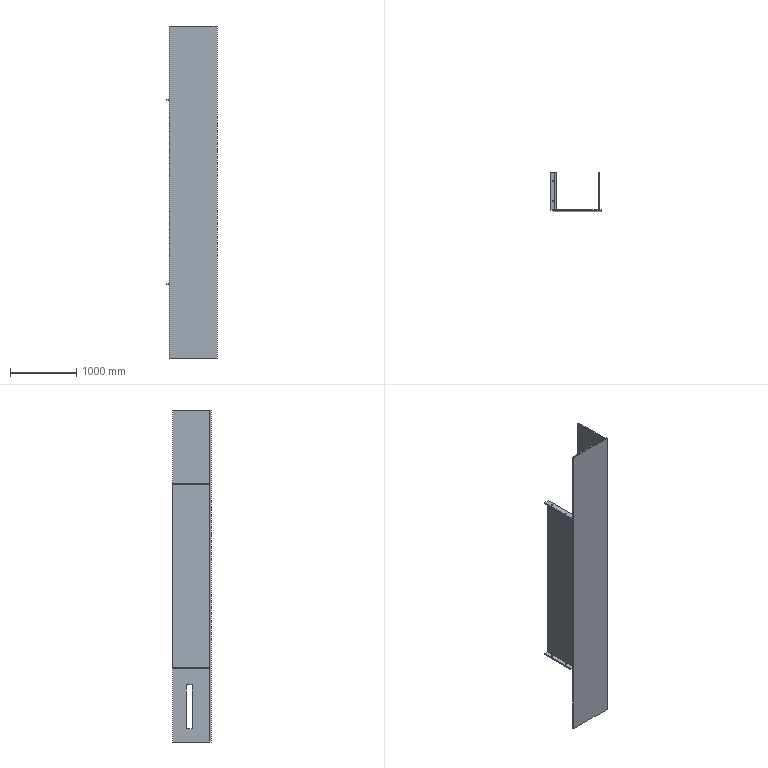Part | SolidWorks | features ICE 4, Extrusion 1 | 1 solid | 34 faces | box 755 x 580 x 5000 mm | volume 159485589 mm3 | plane 26 | cylinder 8 | commonest cylinder face diameters 22 x8
STEP:
#1=CARTESIAN_POINT('',(-376.,450.,3880.));
#2=VERTEX_POINT('',#1);
#3=CARTESIAN_POINT('',(-354.,450.,3880.));
#4=VERTEX_POINT('',#3);
#5=CARTESIAN_POINT('',(-365.,450.,3880.));
#6=DIRECTION('',(0.,0.,1.));
#7=DIRECTION('',(1.,0.,0.));
#8=AXIS2_PLACEMENT_3D('',#5,#6,#7);
#9=CIRCLE('',#8,11.);
#10=EDGE_CURVE('',#2,#4,#9,.T.);
#11=ORIENTED_EDGE('',*,*,#10,.F.);
#12=CARTESIAN_POINT('',(-376.,450.,3900.));
#13=VERTEX_POINT('',#12);
#14=CARTESIAN_POINT('',(-376.,450.,0.));
#15=DIRECTION('',(0.,0.,1.));
#16=VECTOR('',#15,1000.);
#17=LINE('',#14,#16);
#18=EDGE_CURVE('',#2,#13,#17,.T.);
#19=ORIENTED_EDGE('',*,*,#18,.T.);
#20=CARTESIAN_POINT('',(-354.,450.,3900.));
#21=VERTEX_POINT('',#20);
#22=CARTESIAN_POINT('',(-365.,450.,3900.));
#23=DIRECTION('',(0.,0.,1.));
#24=DIRECTION('',(1.,0.,0.));
#25=AXIS2_PLACEMENT_3D('',#22,#23,#24);
#26=CIRCLE('',#25,11.);
#27=EDGE_CURVE('',#13,#21,#26,.T.);
#28=ORIENTED_EDGE('',*,*,#27,.T.);
#29=CARTESIAN_POINT('',(-354.,450.,0.));
#30=DIRECTION('',(0.,0.,1.));
#31=VECTOR('',#30,1000.);
#32=LINE('',#29,#31);
#33=EDGE_CURVE('',#4,#21,#32,.T.);
#34=ORIENTED_EDGE('',*,*,#33,.F.);
#35=EDGE_LOOP('',(#11,#19,#28,#34));
#36=FACE_OUTER_BOUND('',#35,.T.);
#37=CARTESIAN_POINT('',(-365.,450.,0.));
#38=DIRECTION('',(0.,0.,1.));
#39=DIRECTION('',(1.,0.,0.));
#40=AXIS2_PLACEMENT_3D('',#37,#38,#39);
#41=CYLINDRICAL_SURFACE('',#40,11.);
#42=ADVANCED_FACE('',(#36),#41,.F.);
#43=CARTESIAN_POINT('',(-376.,150.,3880.));
#44=VERTEX_POINT('',#43);
#45=CARTESIAN_POINT('',(-354.,150.,3880.));
#46=VERTEX_POINT('',#45);
#47=CARTESIAN_POINT('',(-365.,150.,3880.));
#48=DIRECTION('',(0.,0.,1.));
#49=DIRECTION('',(1.,0.,0.));
#50=AXIS2_PLACEMENT_3D('',#47,#48,#49);
#51=CIRCLE('',#50,11.);
#52=EDGE_CURVE('',#44,#46,#51,.T.);
#53=ORIENTED_EDGE('',*,*,#52,.F.);
#54=CARTESIAN_POINT('',(-376.,150.,3900.));
#55=VERTEX_POINT('',#54);
#56=CARTESIAN_POINT('',(-376.,150.,0.));
#57=DIRECTION('',(0.,0.,1.));
#58=VECTOR('',#57,1000.);
#59=LINE('',#56,#58);
#60=EDGE_CURVE('',#44,#55,#59,.T.);
#61=ORIENTED_EDGE('',*,*,#60,.T.);
#62=CARTESIAN_POINT('',(-354.,150.,3900.));
#63=VERTEX_POINT('',#62);
#64=CARTESIAN_POINT('',(-365.,150.,3900.));
#65=DIRECTION('',(0.,0.,1.));
#66=DIRECTION('',(1.,0.,0.));
#67=AXIS2_PLACEMENT_3D('',#64,#65,#66);
#68=CIRCLE('',#67,11.);
#69=EDGE_CURVE('',#55,#63,#68,.T.);
#70=ORIENTED_EDGE('',*,*,#69,.T.);
#71=CARTESIAN_POINT('',(-354.,150.,0.));
#72=DIRECTION('',(0.,0.,1.));
#73=VECTOR('',#72,1000.);
#74=LINE('',#71,#73);
#75=EDGE_CURVE('',#46,#63,#74,.T.);
#76=ORIENTED_EDGE('',*,*,#75,.F.);
#77=EDGE_LOOP('',(#53,#61,#70,#76));
#78=FACE_OUTER_BOUND('',#77,.T.);
#79=CARTESIAN_POINT('',(-365.,150.,0.));
#80=DIRECTION('',(0.,0.,1.));
#81=DIRECTION('',(1.,0.,0.));
#82=AXIS2_PLACEMENT_3D('',#79,#80,#81);
#83=CYLINDRICAL_SURFACE('',#82,11.);
#84=ADVANCED_FACE('',(#78),#83,.F.);
#85=CARTESIAN_POINT('',(-376.,450.,1100.));
#86=VERTEX_POINT('',#85);
#87=CARTESIAN_POINT('',(-354.,450.,1100.));
#88=VERTEX_POINT('',#87);
#89=CARTESIAN_POINT('',(-365.,450.,1100.));
#90=DIRECTION('',(0.,0.,1.));
#91=DIRECTION('',(1.,0.,0.));
#92=AXIS2_PLACEMENT_3D('',#89,#90,#91);
#93=CIRCLE('',#92,11.);
#94=EDGE_CURVE('',#86,#88,#93,.T.);
#95=ORIENTED_EDGE('',*,*,#94,.F.);
#96=CARTESIAN_POINT('',(-376.,450.,1120.));
#97=VERTEX_POINT('',#96);
#98=CARTESIAN_POINT('',(-376.,450.,0.));
#99=DIRECTION('',(0.,0.,1.));
#100=VECTOR('',#99,1000.);
#101=LINE('',#98,#100);
#102=EDGE_CURVE('',#86,#97,#101,.T.);
#103=ORIENTED_EDGE('',*,*,#102,.T.);
#104=CARTESIAN_POINT('',(-354.,450.,1120.));
#105=VERTEX_POINT('',#104);
#106=CARTESIAN_POINT('',(-365.,450.,1120.));
#107=DIRECTION('',(0.,0.,-1.));
#108=DIRECTION('',(-1.,0.,0.));
#109=AXIS2_PLACEMENT_3D('',#106,#107,#108);
#110=CIRCLE('',#109,11.);
#111=EDGE_CURVE('',#105,#97,#110,.T.);
#112=ORIENTED_EDGE('',*,*,#111,.F.);
#113=CARTESIAN_POINT('',(-354.,450.,0.));
#114=DIRECTION('',(0.,0.,1.));
#115=VECTOR('',#114,1000.);
#116=LINE('',#113,#115);
#117=EDGE_CURVE('',#88,#105,#116,.T.);
#118=ORIENTED_EDGE('',*,*,#117,.F.);
#119=EDGE_LOOP('',(#95,#103,#112,#118));
#120=FACE_OUTER_BOUND('',#119,.T.);
#121=CARTESIAN_POINT('',(-365.,450.,0.));
#122=DIRECTION('',(0.,0.,1.));
#123=DIRECTION('',(1.,0.,0.));
#124=AXIS2_PLACEMENT_3D('',#121,#122,#123);
#125=CYLINDRICAL_SURFACE('',#124,11.);
#126=ADVANCED_FACE('',(#120),#125,.F.);
#127=CARTESIAN_POINT('',(-376.,150.,1100.));
#128=VERTEX_POINT('',#127);
#129=CARTESIAN_POINT('',(-354.,150.,1100.));
#130=VERTEX_POINT('',#129);
#131=CARTESIAN_POINT('',(-365.,150.,1100.));
#132=DIRECTION('',(0.,0.,1.));
#133=DIRECTION('',(1.,0.,0.));
#134=AXIS2_PLACEMENT_3D('',#131,#132,#133);
#135=CIRCLE('',#134,11.);
#136=EDGE_CURVE('',#128,#130,#135,.T.);
#137=ORIENTED_EDGE('',*,*,#136,.F.);
#138=CARTESIAN_POINT('',(-376.,150.,1120.));
#139=VERTEX_POINT('',#138);
#140=CARTESIAN_POINT('',(-376.,150.,0.));
#141=DIRECTION('',(0.,0.,1.));
#142=VECTOR('',#141,1000.);
#143=LINE('',#140,#142);
#144=EDGE_CURVE('',#128,#139,#143,.T.);
#145=ORIENTED_EDGE('',*,*,#144,.T.);
#146=CARTESIAN_POINT('',(-354.,150.,1120.));
#147=VERTEX_POINT('',#146);
#148=CARTESIAN_POINT('',(-365.,150.,1120.));
#149=DIRECTION('',(0.,0.,-1.));
#150=DIRECTION('',(-1.,0.,0.));
#151=AXIS2_PLACEMENT_3D('',#148,#149,#150);
#152=CIRCLE('',#151,11.);
#153=EDGE_CURVE('',#147,#139,#152,.T.);
#154=ORIENTED_EDGE('',*,*,#153,.F.);
#155=CARTESIAN_POINT('',(-354.,150.,0.));
#156=DIRECTION('',(0.,0.,1.));
#157=VECTOR('',#156,1000.);
#158=LINE('',#155,#157);
#159=EDGE_CURVE('',#130,#147,#158,.T.);
#160=ORIENTED_EDGE('',*,*,#159,.F.);
#161=EDGE_LOOP('',(#137,#145,#154,#160));
#162=FACE_OUTER_BOUND('',#161,.T.);
#163=CARTESIAN_POINT('',(-365.,150.,0.));
#164=DIRECTION('',(0.,0.,1.));
#165=DIRECTION('',(1.,0.,0.));
#166=AXIS2_PLACEMENT_3D('',#163,#164,#165);
#167=CYLINDRICAL_SURFACE('',#166,11.);
#168=ADVANCED_FACE('',(#162),#167,.F.);
#169=CARTESIAN_POINT('',(-335.,20.,1120.));
#170=VERTEX_POINT('',#169);
#171=CARTESIAN_POINT('',(-335.,580.,1120.));
#172=VERTEX_POINT('',#171);
#173=CARTESIAN_POINT('',(-335.,580.,1120.));
#174=DIRECTION('',(0.,1.,0.));
#175=VECTOR('',#174,1000.);
#176=LINE('',#173,#175);
#177=EDGE_CURVE('',#170,#172,#176,.T.);
#178=ORIENTED_EDGE('',*,*,#177,.F.);
#179=CARTESIAN_POINT('',(-335.,20.,3880.));
#180=VERTEX_POINT('',#179);
#181=CARTESIAN_POINT('',(-335.,20.,5000.));
#182=DIRECTION('',(0.,0.,-1.));
#183=VECTOR('',#182,1000.);
#184=LINE('',#181,#183);
#185=EDGE_CURVE('',#180,#170,#184,.T.);
#186=ORIENTED_EDGE('',*,*,#185,.F.);
#187=CARTESIAN_POINT('',(-335.,580.,3880.));
#188=VERTEX_POINT('',#187);
#189=CARTESIAN_POINT('',(-335.,580.,3880.));
#190=DIRECTION('',(0.,-1.,0.));
#191=VECTOR('',#190,1000.);
#192=LINE('',#189,#191);
#193=EDGE_CURVE('',#188,#180,#192,.T.);
#194=ORIENTED_EDGE('',*,*,#193,.F.);
#195=CARTESIAN_POINT('',(-335.,580.,5000.));
#196=DIRECTION('',(0.,0.,-1.));
#197=VECTOR('',#196,1000.);
#198=LINE('',#195,#197);
#199=EDGE_CURVE('',#188,#172,#198,.T.);
#200=ORIENTED_EDGE('',*,*,#199,.T.);
#201=EDGE_LOOP('',(#178,#186,#194,#200));
#202=FACE_OUTER_BOUND('',#201,.T.);
#203=CARTESIAN_POINT('',(-335.,20.,5000.));
#204=DIRECTION('',(1.,0.,0.));
#205=DIRECTION('',(0.,1.,0.));
#206=AXIS2_PLACEMENT_3D('',#203,#204,#205);
#207=PLANE('',#206);
#208=ADVANCED_FACE('',(#202),#207,.F.);
#209=CARTESIAN_POINT('',(-360.,20.,1100.));
#210=VERTEX_POINT('',#209);
#211=CARTESIAN_POINT('',(-360.,20.,0.));
#212=VERTEX_POINT('',#211);
#213=CARTESIAN_POINT('',(-360.,20.,5000.));
#214=DIRECTION('',(0.,0.,-1.));
#215=VECTOR('',#214,1000.);
#216=LINE('',#213,#215);
#217=EDGE_CURVE('',#210,#212,#216,.T.);
#218=ORIENTED_EDGE('',*,*,#217,.F.);
#219=CARTESIAN_POINT('',(-315.,20.,1100.));
#220=VERTEX_POINT('',#219);
#221=CARTESIAN_POINT('',(-315.,20.,1100.));
#222=DIRECTION('',(-1.,0.,0.));
#223=VECTOR('',#222,1000.);
#224=LINE('',#221,#223);
#225=EDGE_CURVE('',#220,#210,#224,.T.);
#226=ORIENTED_EDGE('',*,*,#225,.F.);
#227=CARTESIAN_POINT('',(-315.,20.,3900.));
#228=VERTEX_POINT('',#227);
#229=CARTESIAN_POINT('',(-315.,20.,5000.));
#230=DIRECTION('',(0.,0.,-1.));
#231=VECTOR('',#230,1000.);
#232=LINE('',#229,#231);
#233=EDGE_CURVE('',#228,#220,#232,.T.);
#234=ORIENTED_EDGE('',*,*,#233,.F.);
#235=CARTESIAN_POINT('',(-360.,20.,3900.));
#236=VERTEX_POINT('',#235);
#237=CARTESIAN_POINT('',(-315.,20.,3900.));
#238=DIRECTION('',(-1.,0.,0.));
#239=VECTOR('',#238,1000.);
#240=LINE('',#237,#239);
#241=EDGE_CURVE('',#228,#236,#240,.T.);
#242=ORIENTED_EDGE('',*,*,#241,.T.);
#243=CARTESIAN_POINT('',(-360.,20.,5000.));
#244=VERTEX_POINT('',#243);
#245=CARTESIAN_POINT('',(-360.,20.,5000.));
#246=DIRECTION('',(0.,0.,-1.));
#247=VECTOR('',#246,1000.);
#248=LINE('',#245,#247);
#249=EDGE_CURVE('',#244,#236,#248,.T.);
#250=ORIENTED_EDGE('',*,*,#249,.F.);
#251=CARTESIAN_POINT('',(315.,20.,5000.));
#252=VERTEX_POINT('',#251);
#253=CARTESIAN_POINT('',(-315.,20.,5000.));
#254=DIRECTION('',(-1.,0.,0.));
#255=VECTOR('',#254,1000.);
#256=LINE('',#253,#255);
#257=EDGE_CURVE('',#252,#244,#256,.T.);
#258=ORIENTED_EDGE('',*,*,#257,.F.);
#259=CARTESIAN_POINT('',(315.,20.,0.));
#260=VERTEX_POINT('',#259);
#261=CARTESIAN_POINT('',(315.,20.,5000.));
#262=DIRECTION('',(0.,0.,-1.));
#263=VECTOR('',#262,1000.);
#264=LINE('',#261,#263);
#265=EDGE_CURVE('',#252,#260,#264,.T.);
#266=ORIENTED_EDGE('',*,*,#265,.T.);
#267=CARTESIAN_POINT('',(-360.,20.,0.));
#268=DIRECTION('',(-1.,0.,0.));
#269=VECTOR('',#268,1000.);
#270=LINE('',#267,#269);
#271=EDGE_CURVE('',#260,#212,#270,.T.);
#272=ORIENTED_EDGE('',*,*,#271,.T.);
#273=EDGE_LOOP('',(#218,#226,#234,#242,#250,#258,#266,#272));
#274=FACE_OUTER_BOUND('',#273,.T.);
#275=CARTESIAN_POINT('',(-360.,20.,5000.));
#276=DIRECTION('',(0.,-1.,0.));
#277=DIRECTION('',(1.,0.,0.));
#278=AXIS2_PLACEMENT_3D('',#275,#276,#277);
#279=PLANE('',#278);
#280=ADVANCED_FACE('',(#274),#279,.F.);
#281=CARTESIAN_POINT('',(-360.,20.,1120.));
#282=VERTEX_POINT('',#281);
#283=CARTESIAN_POINT('',(-395.,20.,1120.));
#284=DIRECTION('',(1.,0.,0.));
#285=VECTOR('',#284,1000.);
#286=LINE('',#283,#285);
#287=EDGE_CURVE('',#282,#170,#286,.T.);
#288=ORIENTED_EDGE('',*,*,#287,.F.);
#289=CARTESIAN_POINT('',(-360.,20.,3880.));
#290=VERTEX_POINT('',#289);
#291=CARTESIAN_POINT('',(-360.,20.,5000.));
#292=DIRECTION('',(0.,0.,-1.));
#293=VECTOR('',#292,1000.);
#294=LINE('',#291,#293);
#295=EDGE_CURVE('',#290,#282,#294,.T.);
#296=ORIENTED_EDGE('',*,*,#295,.F.);
#297=CARTESIAN_POINT('',(-395.,20.,3880.));
#298=DIRECTION('',(1.,0.,0.));
#299=VECTOR('',#298,1000.);
#300=LINE('',#297,#299);
#301=EDGE_CURVE('',#290,#180,#300,.T.);
#302=ORIENTED_EDGE('',*,*,#301,.T.);
#303=ORIENTED_EDGE('',*,*,#185,.T.);
#304=EDGE_LOOP('',(#288,#296,#302,#303));
#305=FACE_OUTER_BOUND('',#304,.T.);
#306=CARTESIAN_POINT('',(-360.,20.,5000.));
#307=DIRECTION('',(0.,-1.,0.));
#308=DIRECTION('',(1.,0.,0.));
#309=AXIS2_PLACEMENT_3D('',#306,#307,#308);
#310=PLANE('',#309);
#311=ADVANCED_FACE('',(#305),#310,.F.);
#312=CARTESIAN_POINT('',(335.,580.,0.));
#313=VERTEX_POINT('',#312);
#314=CARTESIAN_POINT('',(315.,580.,0.));
#315=VERTEX_POINT('',#314);
#316=CARTESIAN_POINT('',(335.,580.,0.));
#317=DIRECTION('',(-1.,0.,0.));
#318=VECTOR('',#317,1000.);
#319=LINE('',#316,#318);
#320=EDGE_CURVE('',#313,#315,#319,.T.);
#321=ORIENTED_EDGE('',*,*,#320,.T.);
#322=CARTESIAN_POINT('',(315.,580.,5000.));
#323=VERTEX_POINT('',#322);
#324=CARTESIAN_POINT('',(315.,580.,5000.));
#325=DIRECTION('',(0.,0.,-1.));
#326=VECTOR('',#325,1000.);
#327=LINE('',#324,#326);
#328=EDGE_CURVE('',#323,#315,#327,.T.);
#329=ORIENTED_EDGE('',*,*,#328,.F.);
#330=CARTESIAN_POINT('',(335.,580.,5000.));
#331=VERTEX_POINT('',#330);
#332=CARTESIAN_POINT('',(335.,580.,5000.));
#333=DIRECTION('',(-1.,0.,0.));
#334=VECTOR('',#333,1000.);
#335=LINE('',#332,#334);
#336=EDGE_CURVE('',#331,#323,#335,.T.);
#337=ORIENTED_EDGE('',*,*,#336,.F.);
#338=CARTESIAN_POINT('',(335.,580.,5000.));
#339=DIRECTION('',(0.,0.,-1.));
#340=VECTOR('',#339,1000.);
#341=LINE('',#338,#340);
#342=EDGE_CURVE('',#331,#313,#341,.T.);
#343=ORIENTED_EDGE('',*,*,#342,.T.);
#344=EDGE_LOOP('',(#321,#329,#337,#343));
#345=FACE_OUTER_BOUND('',#344,.T.);
#346=CARTESIAN_POINT('',(335.,580.,5000.));
#347=DIRECTION('',(0.,-1.,0.));
#348=DIRECTION('',(0.,0.,-1.));
#349=AXIS2_PLACEMENT_3D('',#346,#347,#348);
#350=PLANE('',#349);
#351=ADVANCED_FACE('',(#345),#350,.F.);
#352=CARTESIAN_POINT('',(315.,285.,200.));
#353=VERTEX_POINT('',#352);
#354=CARTESIAN_POINT('',(315.,285.,860.));
#355=VERTEX_POINT('',#354);
#356=CARTESIAN_POINT('',(315.,285.,860.));
#357=DIRECTION('',(0.,0.,1.));
#358=VECTOR('',#357,1000.);
#359=LINE('',#356,#358);
#360=EDGE_CURVE('',#353,#355,#359,.T.);
#361=ORIENTED_EDGE('',*,*,#360,.F.);
#362=CARTESIAN_POINT('',(315.,375.,200.));
#363=VERTEX_POINT('',#362);
#364=CARTESIAN_POINT('',(315.,375.,200.));
#365=DIRECTION('',(0.,-1.,0.));
#366=VECTOR('',#365,1000.);
#367=LINE('',#364,#366);
#368=EDGE_CURVE('',#363,#353,#367,.T.);
#369=ORIENTED_EDGE('',*,*,#368,.F.);
#370=CARTESIAN_POINT('',(315.,375.,860.));
#371=VERTEX_POINT('',#370);
#372=CARTESIAN_POINT('',(315.,375.,860.));
#373=DIRECTION('',(0.,0.,-1.));
#374=VECTOR('',#373,1000.);
#375=LINE('',#372,#374);
#376=EDGE_CURVE('',#371,#363,#375,.T.);
#377=ORIENTED_EDGE('',*,*,#376,.F.);
#378=CARTESIAN_POINT('',(315.,375.,860.));
#379=DIRECTION('',(0.,1.,0.));
#380=VECTOR('',#379,1000.);
#381=LINE('',#378,#380);
#382=EDGE_CURVE('',#355,#371,#381,.T.);
#383=ORIENTED_EDGE('',*,*,#382,.F.);
#384=EDGE_LOOP('',(#361,#369,#377,#383));
#385=FACE_BOUND('',#384,.T.);
#386=CARTESIAN_POINT('',(315.,580.,0.));
#387=DIRECTION('',(0.,-1.,0.));
#388=VECTOR('',#387,1000.);
#389=LINE('',#386,#388);
#390=EDGE_CURVE('',#315,#260,#389,.T.);
#391=ORIENTED_EDGE('',*,*,#390,.T.);
#392=ORIENTED_EDGE('',*,*,#265,.F.);
#393=CARTESIAN_POINT('',(315.,580.,5000.));
#394=DIRECTION('',(0.,-1.,0.));
#395=VECTOR('',#394,1000.);
#396=LINE('',#393,#395);
#397=EDGE_CURVE('',#323,#252,#396,.T.);
#398=ORIENTED_EDGE('',*,*,#397,.F.);
#399=ORIENTED_EDGE('',*,*,#328,.T.);
#400=EDGE_LOOP('',(#391,#392,#398,#399));
#401=FACE_OUTER_BOUND('',#400,.T.);
#402=CARTESIAN_POINT('',(315.,580.,5000.));
#403=DIRECTION('',(1.,0.,0.));
#404=DIRECTION('',(0.,1.,0.));
#405=AXIS2_PLACEMENT_3D('',#402,#403,#404);
#406=PLANE('',#405);
#407=ADVANCED_FACE('',(#385,#401),#406,.F.);
#408=CARTESIAN_POINT('',(-315.,580.,3900.));
#409=VERTEX_POINT('',#408);
#410=CARTESIAN_POINT('',(-315.,580.,1100.));
#411=VERTEX_POINT('',#410);
#412=CARTESIAN_POINT('',(-315.,580.,5000.));
#413=DIRECTION('',(0.,0.,-1.));
#414=VECTOR('',#413,1000.);
#415=LINE('',#412,#414);
#416=EDGE_CURVE('',#409,#411,#415,.T.);
#417=ORIENTED_EDGE('',*,*,#416,.F.);
#418=CARTESIAN_POINT('',(-315.,580.,3900.));
#419=DIRECTION('',(0.,-1.,0.));
#420=VECTOR('',#419,1000.);
#421=LINE('',#418,#420);
#422=EDGE_CURVE('',#409,#228,#421,.T.);
#423=ORIENTED_EDGE('',*,*,#422,.T.);
#424=ORIENTED_EDGE('',*,*,#233,.T.);
#425=CARTESIAN_POINT('',(-315.,580.,1100.));
#426=DIRECTION('',(0.,1.,0.));
#427=VECTOR('',#426,1000.);
#428=LINE('',#425,#427);
#429=EDGE_CURVE('',#220,#411,#428,.T.);
#430=ORIENTED_EDGE('',*,*,#429,.T.);
#431=EDGE_LOOP('',(#417,#423,#424,#430));
#432=FACE_OUTER_BOUND('',#431,.T.);
#433=CARTESIAN_POINT('',(-315.,580.,5000.));
#434=DIRECTION('',(-1.,0.,0.));
#435=DIRECTION('',(0.,-1.,0.));
#436=AXIS2_PLACEMENT_3D('',#433,#434,#435);
#437=PLANE('',#436);
#438=ADVANCED_FACE('',(#432),#437,.F.);
#439=ORIENTED_EDGE('',*,*,#199,.F.);
#440=CARTESIAN_POINT('',(-395.,580.,3880.));
#441=VERTEX_POINT('',#440);
#442=CARTESIAN_POINT('',(-395.,580.,3880.));
#443=DIRECTION('',(1.,0.,0.));
#444=VECTOR('',#443,1000.);
#445=LINE('',#442,#444);
#446=EDGE_CURVE('',#441,#188,#445,.T.);
#447=ORIENTED_EDGE('',*,*,#446,.F.);
#448=CARTESIAN_POINT('',(-395.,580.,3900.));
#449=VERTEX_POINT('',#448);
#450=CARTESIAN_POINT('',(-395.,580.,3900.));
#451=DIRECTION('',(0.,0.,-1.));
#452=VECTOR('',#451,1000.);
#453=LINE('',#450,#452);
#454=EDGE_CURVE('',#449,#441,#453,.T.);
#455=ORIENTED_EDGE('',*,*,#454,.F.);
#456=CARTESIAN_POINT('',(-315.,580.,3900.));
#457=DIRECTION('',(-1.,0.,0.));
#458=VECTOR('',#457,1000.);
#459=LINE('',#456,#458);
#460=EDGE_CURVE('',#409,#449,#459,.T.);
#461=ORIENTED_EDGE('',*,*,#460,.F.);
#462=ORIENTED_EDGE('',*,*,#416,.T.);
#463=CARTESIAN_POINT('',(-395.,580.,1100.));
#464=VERTEX_POINT('',#463);
#465=CARTESIAN_POINT('',(-315.,580.,1100.));
#466=DIRECTION('',(-1.,0.,0.));
#467=VECTOR('',#466,1000.);
#468=LINE('',#465,#467);
#469=EDGE_CURVE('',#411,#464,#468,.T.);
#470=ORIENTED_EDGE('',*,*,#469,.T.);
#471=CARTESIAN_POINT('',(-395.,580.,1120.));
#472=VERTEX_POINT('',#471);
#473=CARTESIAN_POINT('',(-395.,580.,1100.));
#474=DIRECTION('',(0.,0.,-1.));
#475=VECTOR('',#474,1000.);
#476=LINE('',#473,#475);
#477=EDGE_CURVE('',#472,#464,#476,.T.);
#478=ORIENTED_EDGE('',*,*,#477,.F.);
#479=CARTESIAN_POINT('',(-395.,580.,1120.));
#480=DIRECTION('',(1.,0.,0.));
#481=VECTOR('',#480,1000.);
#482=LINE('',#479,#481);
#483=EDGE_CURVE('',#472,#172,#482,.T.);
#484=ORIENTED_EDGE('',*,*,#483,.T.);
#485=EDGE_LOOP('',(#439,#447,#455,#461,#462,#470,#478,#484));
#486=FACE_OUTER_BOUND('',#485,.T.);
#487=CARTESIAN_POINT('',(-335.,580.,5000.));
#488=DIRECTION('',(0.,-1.,0.));
#489=DIRECTION('',(0.,0.,-1.));
#490=AXIS2_PLACEMENT_3D('',#487,#488,#489);
#491=PLANE('',#490);
#492=ADVANCED_FACE('',(#486),#491,.F.);
#493=CARTESIAN_POINT('',(-360.,0.,0.));
#494=VERTEX_POINT('',#493);
#495=CARTESIAN_POINT('',(-360.,0.,0.));
#496=DIRECTION('',(0.,-1.,0.));
#497=VECTOR('',#496,1000.);
#498=LINE('',#495,#497);
#499=EDGE_CURVE('',#212,#494,#498,.T.);
#500=ORIENTED_EDGE('',*,*,#499,.T.);
#501=CARTESIAN_POINT('',(-360.,0.,5000.));
#502=VERTEX_POINT('',#501);
#503=CARTESIAN_POINT('',(-360.,0.,5000.));
#504=DIRECTION('',(0.,0.,-1.));
#505=VECTOR('',#504,1000.);
#506=LINE('',#503,#505);
#507=EDGE_CURVE('',#502,#494,#506,.T.);
#508=ORIENTED_EDGE('',*,*,#507,.F.);
#509=CARTESIAN_POINT('',(-360.,0.,5000.));
#510=DIRECTION('',(0.,-1.,0.));
#511=VECTOR('',#510,1000.);
#512=LINE('',#509,#511);
#513=EDGE_CURVE('',#244,#502,#512,.T.);
#514=ORIENTED_EDGE('',*,*,#513,.F.);
#515=ORIENTED_EDGE('',*,*,#249,.T.);
#516=CARTESIAN_POINT('',(-360.,20.,5000.));
#517=DIRECTION('',(0.,0.,-1.));
#518=VECTOR('',#517,1000.);
#519=LINE('',#516,#518);
#520=EDGE_CURVE('',#236,#290,#519,.T.);
#521=ORIENTED_EDGE('',*,*,#520,.T.);
#522=ORIENTED_EDGE('',*,*,#295,.T.);
#523=CARTESIAN_POINT('',(-360.,20.,5000.));
#524=DIRECTION('',(0.,0.,-1.));
#525=VECTOR('',#524,1000.);
#526=LINE('',#523,#525);
#527=EDGE_CURVE('',#282,#210,#526,.T.);
#528=ORIENTED_EDGE('',*,*,#527,.T.);
#529=ORIENTED_EDGE('',*,*,#217,.T.);
#530=EDGE_LOOP('',(#500,#508,#514,#515,#521,#522,#528,#529));
#531=FACE_OUTER_BOUND('',#530,.T.);
#532=CARTESIAN_POINT('',(-360.,0.,5000.));
#533=DIRECTION('',(1.,0.,0.));
#534=DIRECTION('',(0.,0.,-1.));
#535=AXIS2_PLACEMENT_3D('',#532,#533,#534);
#536=PLANE('',#535);
#537=ADVANCED_FACE('',(#531),#536,.F.);
#538=CARTESIAN_POINT('',(360.,0.,0.));
#539=VERTEX_POINT('',#538);
#540=CARTESIAN_POINT('',(360.,0.,0.));
#541=DIRECTION('',(1.,0.,0.));
#542=VECTOR('',#541,1000.);
#543=LINE('',#540,#542);
#544=EDGE_CURVE('',#494,#539,#543,.T.);
#545=ORIENTED_EDGE('',*,*,#544,.T.);
#546=CARTESIAN_POINT('',(360.,0.,5000.));
#547=VERTEX_POINT('',#546);
#548=CARTESIAN_POINT('',(360.,0.,5000.));
#549=DIRECTION('',(0.,0.,-1.));
#550=VECTOR('',#549,1000.);
#551=LINE('',#548,#550);
#552=EDGE_CURVE('',#547,#539,#551,.T.);
#553=ORIENTED_EDGE('',*,*,#552,.F.);
#554=CARTESIAN_POINT('',(360.,0.,5000.));
#555=DIRECTION('',(1.,0.,0.));
#556=VECTOR('',#555,1000.);
#557=LINE('',#554,#556);
#558=EDGE_CURVE('',#502,#547,#557,.T.);
#559=ORIENTED_EDGE('',*,*,#558,.F.);
#560=ORIENTED_EDGE('',*,*,#507,.T.);
#561=EDGE_LOOP('',(#545,#553,#559,#560));
#562=FACE_OUTER_BOUND('',#561,.T.);
#563=CARTESIAN_POINT('',(360.,0.,5000.));
#564=DIRECTION('',(0.,1.,0.));
#565=DIRECTION('',(0.,0.,1.));
#566=AXIS2_PLACEMENT_3D('',#563,#564,#565);
#567=PLANE('',#566);
#568=ADVANCED_FACE('',(#562),#567,.F.);
#569=CARTESIAN_POINT('',(360.,20.,0.));
#570=VERTEX_POINT('',#569);
#571=CARTESIAN_POINT('',(360.,0.,0.));
#572=DIRECTION('',(0.,1.,0.));
#573=VECTOR('',#572,1000.);
#574=LINE('',#571,#573);
#575=EDGE_CURVE('',#539,#570,#574,.T.);
#576=ORIENTED_EDGE('',*,*,#575,.T.);
#577=CARTESIAN_POINT('',(360.,20.,5000.));
#578=VERTEX_POINT('',#577);
#579=CARTESIAN_POINT('',(360.,20.,5000.));
#580=DIRECTION('',(0.,0.,-1.));
#581=VECTOR('',#580,1000.);
#582=LINE('',#579,#581);
#583=EDGE_CURVE('',#578,#570,#582,.T.);
#584=ORIENTED_EDGE('',*,*,#583,.F.);
#585=CARTESIAN_POINT('',(360.,0.,5000.));
#586=DIRECTION('',(0.,1.,0.));
#587=VECTOR('',#586,1000.);
#588=LINE('',#585,#587);
#589=EDGE_CURVE('',#547,#578,#588,.T.);
#590=ORIENTED_EDGE('',*,*,#589,.F.);
#591=ORIENTED_EDGE('',*,*,#552,.T.);
#592=EDGE_LOOP('',(#576,#584,#590,#591));
#593=FACE_OUTER_BOUND('',#592,.T.);
#594=CARTESIAN_POINT('',(360.,0.,5000.));
#595=DIRECTION('',(-1.,0.,0.));
#596=DIRECTION('',(0.,0.,1.));
#597=AXIS2_PLACEMENT_3D('',#594,#595,#596);
#598=PLANE('',#597);
#599=ADVANCED_FACE('',(#593),#598,.F.);
#600=CARTESIAN_POINT('',(335.,20.,0.));
#601=VERTEX_POINT('',#600);
#602=CARTESIAN_POINT('',(360.,20.,0.));
#603=DIRECTION('',(-1.,0.,0.));
#604=VECTOR('',#603,1000.);
#605=LINE('',#602,#604);
#606=EDGE_CURVE('',#570,#601,#605,.T.);
#607=ORIENTED_EDGE('',*,*,#606,.T.);
#608=CARTESIAN_POINT('',(335.,20.,5000.));
#609=VERTEX_POINT('',#608);
#610=CARTESIAN_POINT('',(335.,20.,5000.));
#611=DIRECTION('',(0.,0.,-1.));
#612=VECTOR('',#611,1000.);
#613=LINE('',#610,#612);
#614=EDGE_CURVE('',#609,#601,#613,.T.);
#615=ORIENTED_EDGE('',*,*,#614,.F.);
#616=CARTESIAN_POINT('',(360.,20.,5000.));
#617=DIRECTION('',(-1.,0.,0.));
#618=VECTOR('',#617,1000.);
#619=LINE('',#616,#618);
#620=EDGE_CURVE('',#578,#609,#619,.T.);
#621=ORIENTED_EDGE('',*,*,#620,.F.);
#622=ORIENTED_EDGE('',*,*,#583,.T.);
#623=EDGE_LOOP('',(#607,#615,#621,#622));
#624=FACE_OUTER_BOUND('',#623,.T.);
#625=CARTESIAN_POINT('',(360.,20.,5000.));
#626=DIRECTION('',(0.,-1.,0.));
#627=DIRECTION('',(1.,0.,0.));
#628=AXIS2_PLACEMENT_3D('',#625,#626,#627);
#629=PLANE('',#628);
#630=ADVANCED_FACE('',(#624),#629,.F.);
#631=CARTESIAN_POINT('',(335.,375.,200.));
#632=VERTEX_POINT('',#631);
#633=CARTESIAN_POINT('',(335.,375.,860.));
#634=VERTEX_POINT('',#633);
#635=CARTESIAN_POINT('',(335.,375.,860.));
#636=DIRECTION('',(0.,0.,1.));
#637=VECTOR('',#636,1000.);
#638=LINE('',#635,#637);
#639=EDGE_CURVE('',#632,#634,#638,.T.);
#640=ORIENTED_EDGE('',*,*,#639,.F.);
#641=CARTESIAN_POINT('',(335.,285.,200.));
#642=VERTEX_POINT('',#641);
#643=CARTESIAN_POINT('',(335.,375.,200.));
#644=DIRECTION('',(0.,1.,0.));
#645=VECTOR('',#644,1000.);
#646=LINE('',#643,#645);
#647=EDGE_CURVE('',#642,#632,#646,.T.);
#648=ORIENTED_EDGE('',*,*,#647,.F.);
#649=CARTESIAN_POINT('',(335.,285.,860.));
#650=VERTEX_POINT('',#649);
#651=CARTESIAN_POINT('',(335.,285.,860.));
#652=DIRECTION('',(0.,0.,-1.));
#653=VECTOR('',#652,1000.);
#654=LINE('',#651,#653);
#655=EDGE_CURVE('',#650,#642,#654,.T.);
#656=ORIENTED_EDGE('',*,*,#655,.F.);
#657=CARTESIAN_POINT('',(335.,375.,860.));
#658=DIRECTION('',(0.,-1.,0.));
#659=VECTOR('',#658,1000.);
#660=LINE('',#657,#659);
#661=EDGE_CURVE('',#634,#650,#660,.T.);
#662=ORIENTED_EDGE('',*,*,#661,.F.);
#663=EDGE_LOOP('',(#640,#648,#656,#662));
#664=FACE_BOUND('',#663,.T.);
#665=CARTESIAN_POINT('',(335.,20.,0.));
#666=DIRECTION('',(0.,1.,0.));
#667=VECTOR('',#666,1000.);
#668=LINE('',#665,#667);
#669=EDGE_CURVE('',#601,#313,#668,.T.);
#670=ORIENTED_EDGE('',*,*,#669,.T.);
#671=ORIENTED_EDGE('',*,*,#342,.F.);
#672=CARTESIAN_POINT('',(335.,20.,5000.));
#673=DIRECTION('',(0.,1.,0.));
#674=VECTOR('',#673,1000.);
#675=LINE('',#672,#674);
#676=EDGE_CURVE('',#609,#331,#675,.T.);
#677=ORIENTED_EDGE('',*,*,#676,.F.);
#678=ORIENTED_EDGE('',*,*,#614,.T.);
#679=EDGE_LOOP('',(#670,#671,#677,#678));
#680=FACE_OUTER_BOUND('',#679,.T.);
#681=CARTESIAN_POINT('',(335.,20.,5000.));
#682=DIRECTION('',(-1.,0.,0.));
#683=DIRECTION('',(0.,-1.,0.));
#684=AXIS2_PLACEMENT_3D('',#681,#682,#683);
#685=PLANE('',#684);
#686=ADVANCED_FACE('',(#664,#680),#685,.F.);
#687=ORIENTED_EDGE('',*,*,#257,.T.);
#688=ORIENTED_EDGE('',*,*,#513,.T.);
#689=ORIENTED_EDGE('',*,*,#558,.T.);
#690=ORIENTED_EDGE('',*,*,#589,.T.);
#691=ORIENTED_EDGE('',*,*,#620,.T.);
#692=ORIENTED_EDGE('',*,*,#676,.T.);
#693=ORIENTED_EDGE('',*,*,#336,.T.);
#694=ORIENTED_EDGE('',*,*,#397,.T.);
#695=EDGE_LOOP('',(#687,#688,#689,#690,#691,#692,#693,#694));
#696=FACE_OUTER_BOUND('',#695,.T.);
#697=CARTESIAN_POINT('',(0.,0.,5000.));
#698=DIRECTION('',(0.,0.,1.));
#699=DIRECTION('',(1.,0.,0.));
#700=AXIS2_PLACEMENT_3D('',#697,#698,#699);
#701=PLANE('',#700);
#702=ADVANCED_FACE('',(#696),#701,.T.);
#703=ORIENTED_EDGE('',*,*,#271,.F.);
#704=ORIENTED_EDGE('',*,*,#390,.F.);
#705=ORIENTED_EDGE('',*,*,#320,.F.);
#706=ORIENTED_EDGE('',*,*,#669,.F.);
#707=ORIENTED_EDGE('',*,*,#606,.F.);
#708=ORIENTED_EDGE('',*,*,#575,.F.);
#709=ORIENTED_EDGE('',*,*,#544,.F.);
#710=ORIENTED_EDGE('',*,*,#499,.F.);
#711=EDGE_LOOP('',(#703,#704,#705,#706,#707,#708,#709,#710));
#712=FACE_OUTER_BOUND('',#711,.T.);
#713=CARTESIAN_POINT('',(0.,0.,0.));
#714=DIRECTION('',(0.,0.,1.));
#715=DIRECTION('',(1.,0.,0.));
#716=AXIS2_PLACEMENT_3D('',#713,#714,#715);
#717=PLANE('',#716);
#718=ADVANCED_FACE('',(#712),#717,.F.);
#719=ORIENTED_EDGE('',*,*,#368,.T.);
#720=CARTESIAN_POINT('',(-360.001,285.,200.));
#721=DIRECTION('',(1.,0.,0.));
#722=VECTOR('',#721,1000.);
#723=LINE('',#720,#722);
#724=EDGE_CURVE('',#353,#642,#723,.T.);
#725=ORIENTED_EDGE('',*,*,#724,.T.);
#726=ORIENTED_EDGE('',*,*,#647,.T.);
#727=CARTESIAN_POINT('',(-360.001,375.,200.));
#728=DIRECTION('',(1.,0.,0.));
#729=VECTOR('',#728,1000.);
#730=LINE('',#727,#729);
#731=EDGE_CURVE('',#363,#632,#730,.T.);
#732=ORIENTED_EDGE('',*,*,#731,.F.);
#733=EDGE_LOOP('',(#719,#725,#726,#732));
#734=FACE_OUTER_BOUND('',#733,.T.);
#735=CARTESIAN_POINT('',(-360.001,375.,200.));
#736=DIRECTION('',(0.,0.,-1.));
#737=DIRECTION('',(0.,1.,0.));
#738=AXIS2_PLACEMENT_3D('',#735,#736,#737);
#739=PLANE('',#738);
#740=ADVANCED_FACE('',(#734),#739,.F.);
#741=ORIENTED_EDGE('',*,*,#360,.T.);
#742=CARTESIAN_POINT('',(-360.001,285.,860.));
#743=DIRECTION('',(1.,0.,0.));
#744=VECTOR('',#743,1000.);
#745=LINE('',#742,#744);
#746=EDGE_CURVE('',#355,#650,#745,.T.);
#747=ORIENTED_EDGE('',*,*,#746,.T.);
#748=ORIENTED_EDGE('',*,*,#655,.T.);
#749=ORIENTED_EDGE('',*,*,#724,.F.);
#750=EDGE_LOOP('',(#741,#747,#748,#749));
#751=FACE_OUTER_BOUND('',#750,.T.);
#752=CARTESIAN_POINT('',(-360.001,285.,860.));
#753=DIRECTION('',(0.,-1.,0.));
#754=DIRECTION('',(1.,0.,0.));
#755=AXIS2_PLACEMENT_3D('',#752,#753,#754);
#756=PLANE('',#755);
#757=ADVANCED_FACE('',(#751),#756,.F.);
#758=ORIENTED_EDGE('',*,*,#382,.T.);
#759=CARTESIAN_POINT('',(-360.001,375.,860.));
#760=DIRECTION('',(1.,0.,0.));
#761=VECTOR('',#760,1000.);
#762=LINE('',#759,#761);
#763=EDGE_CURVE('',#371,#634,#762,.T.);
#764=ORIENTED_EDGE('',*,*,#763,.T.);
#765=ORIENTED_EDGE('',*,*,#661,.T.);
#766=ORIENTED_EDGE('',*,*,#746,.F.);
#767=EDGE_LOOP('',(#758,#764,#765,#766));
#768=FACE_OUTER_BOUND('',#767,.T.);
#769=CARTESIAN_POINT('',(-360.001,375.,860.));
#770=DIRECTION('',(0.,0.,1.));
#771=DIRECTION('',(1.,0.,0.));
#772=AXIS2_PLACEMENT_3D('',#769,#770,#771);
#773=PLANE('',#772);
#774=ADVANCED_FACE('',(#768),#773,.F.);
#775=ORIENTED_EDGE('',*,*,#376,.T.);
#776=ORIENTED_EDGE('',*,*,#731,.T.);
#777=ORIENTED_EDGE('',*,*,#639,.T.);
#778=ORIENTED_EDGE('',*,*,#763,.F.);
#779=EDGE_LOOP('',(#775,#776,#777,#778));
#780=FACE_OUTER_BOUND('',#779,.T.);
#781=CARTESIAN_POINT('',(-360.001,375.,860.));
#782=DIRECTION('',(0.,1.,0.));
#783=DIRECTION('',(-1.,0.,0.));
#784=AXIS2_PLACEMENT_3D('',#781,#782,#783);
#785=PLANE('',#784);
#786=ADVANCED_FACE('',(#780),#785,.F.);
#787=CARTESIAN_POINT('',(-365.,450.,1100.));
#788=DIRECTION('',(0.,0.,1.));
#789=DIRECTION('',(1.,0.,0.));
#790=AXIS2_PLACEMENT_3D('',#787,#788,#789);
#791=CIRCLE('',#790,11.);
#792=EDGE_CURVE('',#88,#86,#791,.T.);
#793=ORIENTED_EDGE('',*,*,#792,.T.);
#794=ORIENTED_EDGE('',*,*,#94,.T.);
#795=EDGE_LOOP('',(#793,#794));
#796=FACE_BOUND('',#795,.T.);
#797=CARTESIAN_POINT('',(-365.,150.,1100.));
#798=DIRECTION('',(0.,0.,1.));
#799=DIRECTION('',(1.,0.,0.));
#800=AXIS2_PLACEMENT_3D('',#797,#798,#799);
#801=CIRCLE('',#800,11.);
#802=EDGE_CURVE('',#130,#128,#801,.T.);
#803=ORIENTED_EDGE('',*,*,#802,.T.);
#804=ORIENTED_EDGE('',*,*,#136,.T.);
#805=EDGE_LOOP('',(#803,#804));
#806=FACE_BOUND('',#805,.T.);
#807=ORIENTED_EDGE('',*,*,#225,.T.);
#808=CARTESIAN_POINT('',(-395.,20.,1100.));
#809=VERTEX_POINT('',#808);
#810=CARTESIAN_POINT('',(-395.,20.,1100.));
#811=DIRECTION('',(1.,0.,0.));
#812=VECTOR('',#811,1000.);
#813=LINE('',#810,#812);
#814=EDGE_CURVE('',#809,#210,#813,.T.);
#815=ORIENTED_EDGE('',*,*,#814,.F.);
#816=CARTESIAN_POINT('',(-395.,580.,1100.));
#817=DIRECTION('',(0.,-1.,0.));
#818=VECTOR('',#817,1000.);
#819=LINE('',#816,#818);
#820=EDGE_CURVE('',#464,#809,#819,.T.);
#821=ORIENTED_EDGE('',*,*,#820,.F.);
#822=ORIENTED_EDGE('',*,*,#469,.F.);
#823=ORIENTED_EDGE('',*,*,#429,.F.);
#824=EDGE_LOOP('',(#807,#815,#821,#822,#823));
#825=FACE_OUTER_BOUND('',#824,.T.);
#826=CARTESIAN_POINT('',(-315.,580.,1100.));
#827=DIRECTION('',(0.,0.,1.));
#828=DIRECTION('',(1.,0.,0.));
#829=AXIS2_PLACEMENT_3D('',#826,#827,#828);
#830=PLANE('',#829);
#831=ADVANCED_FACE('',(#796,#806,#825),#830,.F.);
#832=CARTESIAN_POINT('',(-365.,450.,3900.));
#833=DIRECTION('',(0.,0.,1.));
#834=DIRECTION('',(1.,0.,0.));
#835=AXIS2_PLACEMENT_3D('',#832,#833,#834);
#836=CIRCLE('',#835,11.);
#837=EDGE_CURVE('',#21,#13,#836,.T.);
#838=ORIENTED_EDGE('',*,*,#837,.F.);
#839=ORIENTED_EDGE('',*,*,#27,.F.);
#840=EDGE_LOOP('',(#838,#839));
#841=FACE_BOUND('',#840,.T.);
#842=CARTESIAN_POINT('',(-365.,150.,3900.));
#843=DIRECTION('',(0.,0.,1.));
#844=DIRECTION('',(1.,0.,0.));
#845=AXIS2_PLACEMENT_3D('',#842,#843,#844);
#846=CIRCLE('',#845,11.);
#847=EDGE_CURVE('',#63,#55,#846,.T.);
#848=ORIENTED_EDGE('',*,*,#847,.F.);
#849=ORIENTED_EDGE('',*,*,#69,.F.);
#850=EDGE_LOOP('',(#848,#849));
#851=FACE_BOUND('',#850,.T.);
#852=ORIENTED_EDGE('',*,*,#460,.T.);
#853=CARTESIAN_POINT('',(-395.,20.,3900.));
#854=VERTEX_POINT('',#853);
#855=CARTESIAN_POINT('',(-395.,580.,3900.));
#856=DIRECTION('',(0.,1.,0.));
#857=VECTOR('',#856,1000.);
#858=LINE('',#855,#857);
#859=EDGE_CURVE('',#854,#449,#858,.T.);
#860=ORIENTED_EDGE('',*,*,#859,.F.);
#861=CARTESIAN_POINT('',(-395.,20.,3900.));
#862=DIRECTION('',(1.,0.,0.));
#863=VECTOR('',#862,1000.);
#864=LINE('',#861,#863);
#865=EDGE_CURVE('',#854,#236,#864,.T.);
#866=ORIENTED_EDGE('',*,*,#865,.T.);
#867=ORIENTED_EDGE('',*,*,#241,.F.);
#868=ORIENTED_EDGE('',*,*,#422,.F.);
#869=EDGE_LOOP('',(#852,#860,#866,#867,#868));
#870=FACE_OUTER_BOUND('',#869,.T.);
#871=CARTESIAN_POINT('',(-315.,580.,3900.));
#872=DIRECTION('',(0.,0.,-1.));
#873=DIRECTION('',(-1.,0.,0.));
#874=AXIS2_PLACEMENT_3D('',#871,#872,#873);
#875=PLANE('',#874);
#876=ADVANCED_FACE('',(#841,#851,#870),#875,.F.);
#877=CARTESIAN_POINT('',(-395.,20.,3880.));
#878=VERTEX_POINT('',#877);
#879=CARTESIAN_POINT('',(-395.,20.,3880.));
#880=DIRECTION('',(1.,0.,0.));
#881=VECTOR('',#880,1000.);
#882=LINE('',#879,#881);
#883=EDGE_CURVE('',#878,#290,#882,.T.);
#884=ORIENTED_EDGE('',*,*,#883,.T.);
#885=ORIENTED_EDGE('',*,*,#520,.F.);
#886=ORIENTED_EDGE('',*,*,#865,.F.);
#887=CARTESIAN_POINT('',(-395.,20.,3900.));
#888=DIRECTION('',(0.,0.,1.));
#889=VECTOR('',#888,1000.);
#890=LINE('',#887,#889);
#891=EDGE_CURVE('',#878,#854,#890,.T.);
#892=ORIENTED_EDGE('',*,*,#891,.F.);
#893=EDGE_LOOP('',(#884,#885,#886,#892));
#894=FACE_OUTER_BOUND('',#893,.T.);
#895=CARTESIAN_POINT('',(-395.,20.,3900.));
#896=DIRECTION('',(0.,1.,0.));
#897=DIRECTION('',(-1.,0.,0.));
#898=AXIS2_PLACEMENT_3D('',#895,#896,#897);
#899=PLANE('',#898);
#900=ADVANCED_FACE('',(#894),#899,.F.);
#901=CARTESIAN_POINT('',(-365.,450.,3880.));
#902=DIRECTION('',(0.,0.,1.));
#903=DIRECTION('',(1.,0.,0.));
#904=AXIS2_PLACEMENT_3D('',#901,#902,#903);
#905=CIRCLE('',#904,11.);
#906=EDGE_CURVE('',#4,#2,#905,.T.);
#907=ORIENTED_EDGE('',*,*,#906,.T.);
#908=ORIENTED_EDGE('',*,*,#10,.T.);
#909=EDGE_LOOP('',(#907,#908));
#910=FACE_BOUND('',#909,.T.);
#911=CARTESIAN_POINT('',(-365.,150.,3880.));
#912=DIRECTION('',(0.,0.,1.));
#913=DIRECTION('',(1.,0.,0.));
#914=AXIS2_PLACEMENT_3D('',#911,#912,#913);
#915=CIRCLE('',#914,11.);
#916=EDGE_CURVE('',#46,#44,#915,.T.);
#917=ORIENTED_EDGE('',*,*,#916,.T.);
#918=ORIENTED_EDGE('',*,*,#52,.T.);
#919=EDGE_LOOP('',(#917,#918));
#920=FACE_BOUND('',#919,.T.);
#921=ORIENTED_EDGE('',*,*,#193,.T.);
#922=ORIENTED_EDGE('',*,*,#301,.F.);
#923=ORIENTED_EDGE('',*,*,#883,.F.);
#924=CARTESIAN_POINT('',(-395.,580.,3880.));
#925=DIRECTION('',(0.,-1.,0.));
#926=VECTOR('',#925,1000.);
#927=LINE('',#924,#926);
#928=EDGE_CURVE('',#441,#878,#927,.T.);
#929=ORIENTED_EDGE('',*,*,#928,.F.);
#930=ORIENTED_EDGE('',*,*,#446,.T.);
#931=EDGE_LOOP('',(#921,#922,#923,#929,#930));
#932=FACE_OUTER_BOUND('',#931,.T.);
#933=CARTESIAN_POINT('',(-395.,580.,3880.));
#934=DIRECTION('',(0.,0.,1.));
#935=DIRECTION('',(1.,0.,0.));
#936=AXIS2_PLACEMENT_3D('',#933,#934,#935);
#937=PLANE('',#936);
#938=ADVANCED_FACE('',(#910,#920,#932),#937,.F.);
#939=ORIENTED_EDGE('',*,*,#859,.T.);
#940=ORIENTED_EDGE('',*,*,#454,.T.);
#941=ORIENTED_EDGE('',*,*,#928,.T.);
#942=ORIENTED_EDGE('',*,*,#891,.T.);
#943=EDGE_LOOP('',(#939,#940,#941,#942));
#944=FACE_OUTER_BOUND('',#943,.T.);
#945=CARTESIAN_POINT('',(-395.,0.,0.));
#946=DIRECTION('',(1.,0.,0.));
#947=DIRECTION('',(0.,1.,0.));
#948=AXIS2_PLACEMENT_3D('',#945,#946,#947);
#949=PLANE('',#948);
#950=ADVANCED_FACE('',(#944),#949,.F.);
#951=ORIENTED_EDGE('',*,*,#814,.T.);
#952=ORIENTED_EDGE('',*,*,#527,.F.);
#953=CARTESIAN_POINT('',(-395.,20.,1120.));
#954=VERTEX_POINT('',#953);
#955=CARTESIAN_POINT('',(-395.,20.,1120.));
#956=DIRECTION('',(1.,0.,0.));
#957=VECTOR('',#956,1000.);
#958=LINE('',#955,#957);
#959=EDGE_CURVE('',#954,#282,#958,.T.);
#960=ORIENTED_EDGE('',*,*,#959,.F.);
#961=CARTESIAN_POINT('',(-395.,20.,1100.));
#962=DIRECTION('',(0.,0.,1.));
#963=VECTOR('',#962,1000.);
#964=LINE('',#961,#963);
#965=EDGE_CURVE('',#809,#954,#964,.T.);
#966=ORIENTED_EDGE('',*,*,#965,.F.);
#967=EDGE_LOOP('',(#951,#952,#960,#966));
#968=FACE_OUTER_BOUND('',#967,.T.);
#969=CARTESIAN_POINT('',(-395.,20.,1100.));
#970=DIRECTION('',(0.,1.,0.));
#971=DIRECTION('',(0.,0.,1.));
#972=AXIS2_PLACEMENT_3D('',#969,#970,#971);
#973=PLANE('',#972);
#974=ADVANCED_FACE('',(#968),#973,.F.);
#975=ORIENTED_EDGE('',*,*,#111,.T.);
#976=CARTESIAN_POINT('',(-365.,450.,1120.));
#977=DIRECTION('',(0.,0.,-1.));
#978=DIRECTION('',(-1.,0.,0.));
#979=AXIS2_PLACEMENT_3D('',#976,#977,#978);
#980=CIRCLE('',#979,11.);
#981=EDGE_CURVE('',#97,#105,#980,.T.);
#982=ORIENTED_EDGE('',*,*,#981,.T.);
#983=EDGE_LOOP('',(#975,#982));
#984=FACE_BOUND('',#983,.T.);
#985=ORIENTED_EDGE('',*,*,#153,.T.);
#986=CARTESIAN_POINT('',(-365.,150.,1120.));
#987=DIRECTION('',(0.,0.,-1.));
#988=DIRECTION('',(-1.,0.,0.));
#989=AXIS2_PLACEMENT_3D('',#986,#987,#988);
#990=CIRCLE('',#989,11.);
#991=EDGE_CURVE('',#139,#147,#990,.T.);
#992=ORIENTED_EDGE('',*,*,#991,.T.);
#993=EDGE_LOOP('',(#985,#992));
#994=FACE_BOUND('',#993,.T.);
#995=ORIENTED_EDGE('',*,*,#177,.T.);
#996=ORIENTED_EDGE('',*,*,#483,.F.);
#997=CARTESIAN_POINT('',(-395.,580.,1120.));
#998=DIRECTION('',(0.,1.,0.));
#999=VECTOR('',#998,1000.);
#1000=LINE('',#997,#999);
#1001=EDGE_CURVE('',#954,#472,#1000,.T.);
#1002=ORIENTED_EDGE('',*,*,#1001,.F.);
#1003=ORIENTED_EDGE('',*,*,#959,.T.);
#1004=ORIENTED_EDGE('',*,*,#287,.T.);
#1005=EDGE_LOOP('',(#995,#996,#1002,#1003,#1004));
#1006=FACE_OUTER_BOUND('',#1005,.T.);
#1007=CARTESIAN_POINT('',(-395.,580.,1120.));
#1008=DIRECTION('',(0.,0.,-1.));
#1009=DIRECTION('',(-1.,0.,0.));
#1010=AXIS2_PLACEMENT_3D('',#1007,#1008,#1009);
#1011=PLANE('',#1010);
#1012=ADVANCED_FACE('',(#984,#994,#1006),#1011,.F.);
#1013=ORIENTED_EDGE('',*,*,#820,.T.);
#1014=ORIENTED_EDGE('',*,*,#965,.T.);
#1015=ORIENTED_EDGE('',*,*,#1001,.T.);
#1016=ORIENTED_EDGE('',*,*,#477,.T.);
#1017=EDGE_LOOP('',(#1013,#1014,#1015,#1016));
#1018=FACE_OUTER_BOUND('',#1017,.T.);
#1019=CARTESIAN_POINT('',(-395.,0.,0.));
#1020=DIRECTION('',(-1.,0.,0.));
#1021=DIRECTION('',(0.,-1.,0.));
#1022=AXIS2_PLACEMENT_3D('',#1019,#1020,#1021);
#1023=PLANE('',#1022);
#1024=ADVANCED_FACE('',(#1018),#1023,.T.);
#1025=ORIENTED_EDGE('',*,*,#144,.F.);
#1026=ORIENTED_EDGE('',*,*,#802,.F.);
#1027=ORIENTED_EDGE('',*,*,#159,.T.);
#1028=ORIENTED_EDGE('',*,*,#991,.F.);
#1029=EDGE_LOOP('',(#1025,#1026,#1027,#1028));
#1030=FACE_OUTER_BOUND('',#1029,.T.);
#1031=CARTESIAN_POINT('',(-365.,150.,0.));
#1032=DIRECTION('',(0.,0.,1.));
#1033=DIRECTION('',(1.,0.,0.));
#1034=AXIS2_PLACEMENT_3D('',#1031,#1032,#1033);
#1035=CYLINDRICAL_SURFACE('',#1034,11.);
#1036=ADVANCED_FACE('',(#1030),#1035,.F.);
#1037=ORIENTED_EDGE('',*,*,#102,.F.);
#1038=ORIENTED_EDGE('',*,*,#792,.F.);
#1039=ORIENTED_EDGE('',*,*,#117,.T.);
#1040=ORIENTED_EDGE('',*,*,#981,.F.);
#1041=EDGE_LOOP('',(#1037,#1038,#1039,#1040));
#1042=FACE_OUTER_BOUND('',#1041,.T.);
#1043=CARTESIAN_POINT('',(-365.,450.,0.));
#1044=DIRECTION('',(0.,0.,1.));
#1045=DIRECTION('',(1.,0.,0.));
#1046=AXIS2_PLACEMENT_3D('',#1043,#1044,#1045);
#1047=CYLINDRICAL_SURFACE('',#1046,11.);
#1048=ADVANCED_FACE('',(#1042),#1047,.F.);
#1049=ORIENTED_EDGE('',*,*,#60,.F.);
#1050=ORIENTED_EDGE('',*,*,#916,.F.);
#1051=ORIENTED_EDGE('',*,*,#75,.T.);
#1052=ORIENTED_EDGE('',*,*,#847,.T.);
#1053=EDGE_LOOP('',(#1049,#1050,#1051,#1052));
#1054=FACE_OUTER_BOUND('',#1053,.T.);
#1055=CARTESIAN_POINT('',(-365.,150.,0.));
#1056=DIRECTION('',(0.,0.,1.));
#1057=DIRECTION('',(1.,0.,0.));
#1058=AXIS2_PLACEMENT_3D('',#1055,#1056,#1057);
#1059=CYLINDRICAL_SURFACE('',#1058,11.);
#1060=ADVANCED_FACE('',(#1054),#1059,.F.);
#1061=ORIENTED_EDGE('',*,*,#18,.F.);
#1062=ORIENTED_EDGE('',*,*,#906,.F.);
#1063=ORIENTED_EDGE('',*,*,#33,.T.);
#1064=ORIENTED_EDGE('',*,*,#837,.T.);
#1065=EDGE_LOOP('',(#1061,#1062,#1063,#1064));
#1066=FACE_OUTER_BOUND('',#1065,.T.);
#1067=CARTESIAN_POINT('',(-365.,450.,0.));
#1068=DIRECTION('',(0.,0.,1.));
#1069=DIRECTION('',(1.,0.,0.));
#1070=AXIS2_PLACEMENT_3D('',#1067,#1068,#1069);
#1071=CYLINDRICAL_SURFACE('',#1070,11.);
#1072=ADVANCED_FACE('',(#1066),#1071,.F.);
#1073=CLOSED_SHELL('',(#42,#84,#126,#168,#208,#280,#311,#351,#407,#438,#492,#537,#568,#599,#630,#686,#702,#718,#740,#757,#774,#786,#831,#876,#900,#938,#950,#974,#1012,#1024,#1036,#1048,#1060,#1072));
#1074=MANIFOLD_SOLID_BREP('',#1073);
#1075=CARTESIAN_POINT('',(0.,0.,0.));
#1076=DIRECTION('',(0.,0.,1.));
#1077=DIRECTION('',(1.,0.,0.));
#1078=AXIS2_PLACEMENT_3D('',#1075,#1076,#1077);
#1079=(LENGTH_UNIT()NAMED_UNIT(*)SI_UNIT(.MILLI.,.METRE.));
#1080=UNCERTAINTY_MEASURE_WITH_UNIT(LENGTH_MEASURE(0.00001),#1079,'','');
#1081=(NAMED_UNIT(*)PLANE_ANGLE_UNIT()SI_UNIT($,.RADIAN.));
#1082=(NAMED_UNIT(*)SI_UNIT($,.STERADIAN.)SOLID_ANGLE_UNIT());
#1083=(GEOMETRIC_REPRESENTATION_CONTEXT(3)GLOBAL_UNCERTAINTY_ASSIGNED_CONTEXT((#1080))GLOBAL_UNIT_ASSIGNED_CONTEXT((#1079,#1081,#1082))REPRESENTATION_CONTEXT('',''));
#1084=ADVANCED_BREP_SHAPE_REPRESENTATION('',(#1074,#1078),#1083);